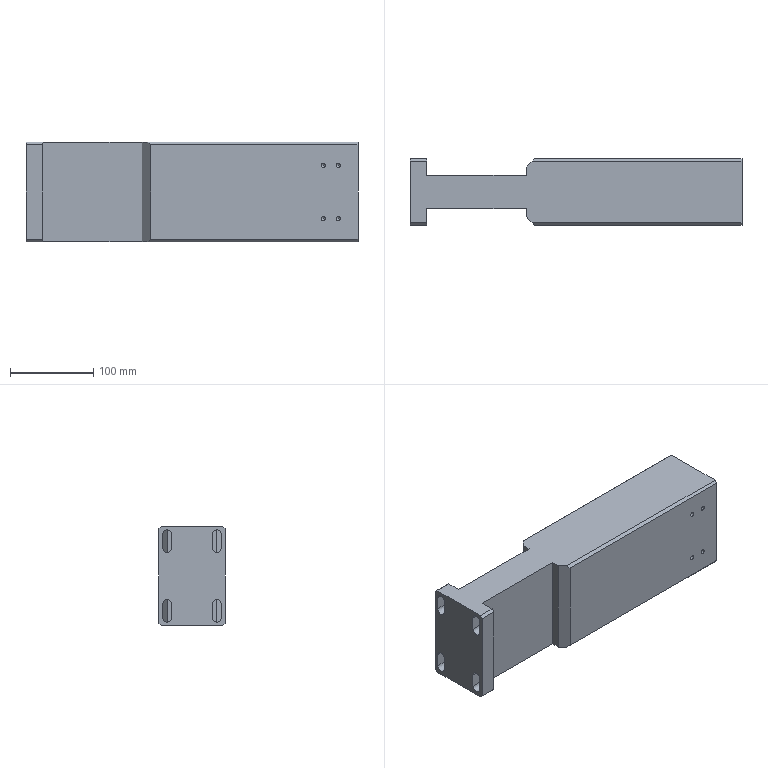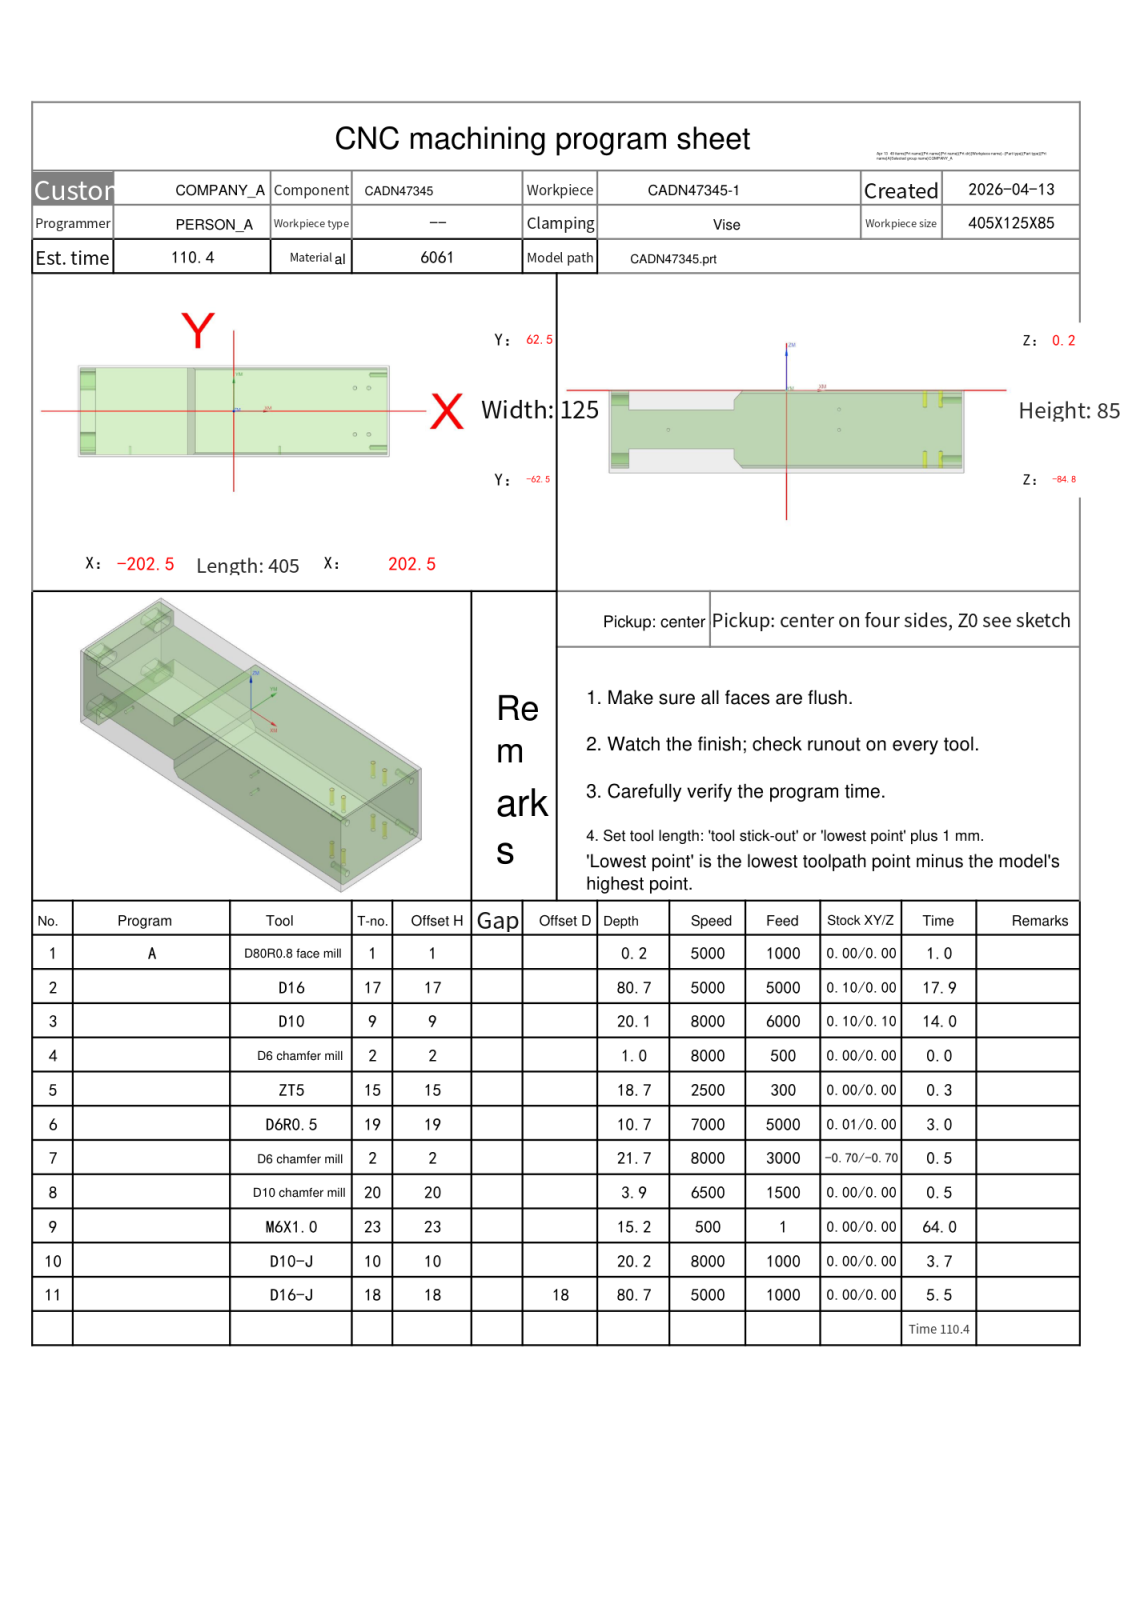NC program | NX | posted by the shop | part box 400 x 80 x 120 mm
Lines 4941 to 5986 of 5986:
N4 T02 M06
(D6 chamfer mill  D=6. R=0. H=02 ce=0.00 di=0.10)
G00 G90 G54 X158. Y32. M03 S8000
G43 H02 Z20.
M08
G98 G81 X158. Y32. Z-.8 R1. F500.
X176.
Y-32.
X158.
G80
G00 Z20.
G91 G28 Z0.0
M05
M09
G91 G28 Z0.0
M01
N5 T15 M06
(ZT5 D=5. DR_a=118 H=15)
G00 G90 G54 X158. Y32. M03 S2500
G43 H15 Z20.
M08
G98 G83 X158. Y32. Z-18.502 R1. F300. Q3.
X176.
Y-32.
X158.
G80
G00 Z20.
G91 G28 Z0.0
M05
M09
G91 G28 Z0.0
M01
N6 T19 M06
(D6R0.5  D=6. R=0.5 H=19 ce=0.01 di=0.00)
G00 G90 G54 X-52.801 Y-63.373 M03 S7000
G43 H19 Z10.788
M08
Z.415
G01 Z-.085 F5000.
Y-58.246
Y58.246
X-52.884 Y58.332 Z-.17
X-52.887 Y58.275
Y-58.275
X-52.884 Y-58.332
X-52.968 Y-58.417 Z-.255
X-52.972 Y-58.275
Y58.275
X-52.968 Y58.417
X-53.053 Y58.503 Z-.339
X-53.057 Y58.275
Y-58.275
X-53.053 Y-58.503
X-53.14 Y-58.588 Z-.424
X-53.141 Y-57.278
Y57.278
X-53.14 Y58.588
X-53.224 Y58.674 Z-.509
X-53.226 Y58.622
Y-58.622
X-53.224 Y-58.674
X-53.308 Y-58.759 Z-.594
X-53.311 Y-58.622
Y58.622
X-53.308 Y58.759
X-53.393 Y58.845 Z-.679
X-53.396 Y58.622
Y-58.622
X-53.393 Y-58.844
X-53.479 Y-58.93 Z-.764
X-53.481 Y-57.617
Y57.617
X-53.479 Y58.93
X-53.563 Y59.015 Z-.849
X-53.566 Y58.969
Y-58.969
X-53.563 Y-59.015
X-53.647 Y-59.099 Z-.933
X-53.65 Y-58.969
Y58.969
X-53.647 Y59.099
X-53.732 Y59.184 Z-1.018
X-53.735 Y58.969
Y-58.969
X-53.732 Y-59.184
X-53.819 Y-59.269 Z-1.103
X-53.82 Y-57.957
Y57.957
X-53.819 Y59.269
X-53.903 Y59.354 Z-1.188
X-53.905 Y59.316
Y-59.316
X-53.903 Y-59.354
X-53.987 Y-59.439 Z-1.273
X-53.99 Y-59.316
Y59.316
X-53.987 Y59.438
X-54.071 Y59.523 Z-1.358
X-54.075 Y59.316
Y-59.316
X-54.071 Y-59.523
X-54.158 Y-59.608 Z-1.442
X-54.16 Y-58.296
Y58.296
X-54.158 Y59.608
X-54.243 Y59.693 Z-1.527
X-54.244 Y59.663
Y-59.663
X-54.243 Y-59.693
X-54.326 Y-59.777 Z-1.612
X-54.329 Y-59.663
Y59.663
X-54.326 Y59.777
X-54.411 Y59.862 Z-1.697
X-54.414 Y59.663
Y-59.663
X-54.411 Y-59.862
X-54.497 Y-59.946 Z-1.782
X-54.499 Y-58.635
Y58.635
X-54.497 Y59.946
X-54.583 Y60.03 Z-1.867
X-54.584 Y58.72
Y-58.72
X-54.583 Y-60.03
X-54.666 Y-60.114 Z-1.952
X-54.669 Y-60.009
Y60.009
X-54.666 Y60.114
X-54.75 Y60.198 Z-2.036
X-54.754 Y60.009
Y-60.009
X-54.75 Y-60.198
X-54.836 Y-60.282 Z-2.121
X-54.838 Y-58.975
Y58.975
X-54.836 Y60.282
X-54.923 Y60.366 Z-2.206
Y59.06
Y-59.06
Y-60.366
X-55.005 Y-60.45 Z-2.291
X-55.008 Y-60.356
Y60.356
X-55.005 Y60.45
X-55.089 Y60.534 Z-2.376
X-55.093 Y60.356
Y-60.356
X-55.089 Y-60.534
X-55.175 Y-60.618 Z-2.461
X-55.178 Y-59.314
Y59.314
X-55.175 Y60.618
X-55.263 Y60.703 Z-2.546
Y59.399
Y-59.399
Y-60.703
X-55.346 Y-60.786 Z-2.63
X-55.348 Y-60.703
Y60.703
X-55.346 Y60.786
X-55.429 Y60.87 Z-2.715
X-55.432 Y60.703
Y-60.703
X-55.429 Y-60.87
X-55.514 Y-60.954 Z-2.8
X-55.517 Y-60.703
Y60.703
X-55.514 Y60.954
X-55.602 Y61.038 Z-2.885
Y59.739
Y-59.739
Y-61.038
X-55.645 Y-61.05 Z-2.927
X-55.686 Y-61.061 Z-2.97
X-55.687 Y-59.823
Y59.823
X-55.686 Y61.061
X-55.729 Y61.062 Z-3.012
X-55.771 Z-3.055
X-55.772 Y59.908
Y-59.908
X-55.771 Y-61.063
X-55.814 Z-3.097
X-55.856 Z-3.14
X-55.857 Y-59.993
Y59.993
X-55.856 Y61.063
X-55.899 Y61.064 Z-3.182
X-55.941 Z-3.224
X-55.942 Y60.
Y-60.
X-55.941 Y-61.064
X-55.984 Y-61.065 Z-3.267
X-56.026 Z-3.309
Y-60.
Y60.
Y61.065
X-56.069 Y61.066 Z-3.352
X-56.11 Z-3.394
X-56.111 Y60.
Y-60.
X-56.11 Y-61.066
X-56.154 Z-3.437
X-56.195 Y-61.067 Z-3.479
X-56.196 Y-60.
Y60.
X-56.195 Y61.067
X-56.238 Z-3.521
X-56.28 Y61.068 Z-3.564
X-56.281 Y60.
Y-60.
X-56.28 Y-61.068
X-56.323 Z-3.606
X-56.365 Y-61.069 Z-3.649
X-56.366 Y-60.
Y60.
X-56.365 Y61.069
X-56.408 Z-3.691
X-56.45 Y61.07 Z-3.734
X-56.451 Y60.
Y-60.
X-56.45 Y-61.069
X-56.493 Y-61.07 Z-3.776
X-56.534 Z-3.818
X-56.535 Y-60.
Y60.
X-56.534 Y61.07
X-56.578 Y61.071 Z-3.861
X-56.619 Z-3.903
X-56.62 Y60.
Y-60.
X-56.619 Y-61.071
X-56.663 Y-61.072 Z-3.946
X-56.704 Z-3.988
X-56.705 Y-60.
Y60.
X-56.704 Y61.072
X-56.748 Y61.073 Z-4.031
X-56.789 Z-4.073
X-56.79 Y60.
Y-60.
X-56.789 Y-61.073
X-56.832 Y-61.074 Z-4.115
X-56.874 Z-4.158
X-56.875 Y-60.
Y60.
X-56.874 Y61.074
X-56.917 Z-4.2
X-56.958 Y61.075 Z-4.243
X-56.96 Y61.05
Y-61.05
X-56.958 Y-61.075
X-57.002 Z-4.285
X-57.043 Y-61.076 Z-4.327
X-57.045 Y-61.05
Y61.05
X-57.043 Y61.076
X-57.087 Z-4.37
X-57.128 Y61.077 Z-4.412
X-57.129 Y61.05
Y-61.05
X-57.128 Y-61.077
X-57.172 Z-4.455
X-57.211 Z-4.497
X-57.212 Y-61.05
Y61.05
X-57.211 Y61.077
X-57.257 Y61.078 Z-4.54
X-57.298 Z-4.582
X-57.299 Y61.05
Y-61.05
X-57.298 Y-61.078
X-57.342 Y-61.079 Z-4.624
X-57.383 Z-4.667
X-57.384 Y-61.05
Y61.05
X-57.383 Y61.079
X-57.426 Z-4.709
X-57.467 Z-4.752
X-57.469 Y61.05
Y-61.05
X-57.467 Y-61.08
X-57.511 Z-4.794
X-57.552 Z-4.837
X-57.554 Y-61.05
Y61.05
X-57.552 Y61.08
X-57.596 Z-4.879
X-57.637 Y61.081 Z-4.921
X-57.639 Y61.05
Y-61.05
X-57.637 Y-61.081
X-57.681 Z-4.964
X-57.722 Z-5.006
X-57.723 Y-61.05
Y61.05
X-57.722 Y61.081
X-57.766 Y61.082 Z-5.049
X-57.807 Z-5.091
X-57.808 Y61.05
Y-61.05
X-57.807 Y-61.082
X-57.851 Z-5.134
X-57.892 Z-5.176
X-57.893 Y-61.05
Y61.05
X-57.892 Y61.082
X-57.936 Y61.083 Z-5.218
X-57.976 Z-5.261
X-57.978 Y61.05
Y-61.05
X-57.976 Y-61.083
X-58.02 Z-5.303
X-58.061 Y-61.084 Z-5.346
X-58.063 Y-61.05
Y61.05
X-58.061 Y61.084
X-58.105 Z-5.388
X-58.146 Z-5.431
X-58.148 Y61.05
Y-61.05
X-58.146 Y-61.084
X-58.19 Y-61.085 Z-5.473
X-58.231 Z-5.515
X-58.233 Y-61.05
Y61.05
X-58.231 Y61.085
X-58.275 Z-5.558
X-58.316 Z-5.6
X-58.317 Y61.05
Y-61.05
X-58.316 Y-61.085
X-58.36 Y-61.086 Z-5.643
X-58.4 Z-5.685
X-58.402 Y-61.05
Y61.05
X-58.401 Y61.086
X-58.445 Z-5.728
X-58.485 Z-5.77
X-58.487 Y61.05
Y-61.05
X-58.485 Y-61.086
X-58.53 Y-61.087 Z-5.812
X-58.57 Z-5.855
X-58.572 Y-61.05
Y61.05
X-58.57 Y61.087
X-58.614 Z-5.897
X-58.655 Z-5.94
X-58.657 Y61.05
Y-61.05
X-58.655 Y-61.087
X-58.699 Z-5.982
X-58.74 Z-6.025
X-58.742 Y-61.05
Y61.05
X-58.74 Y61.088
X-58.784 Z-6.067
X-58.825 Z-6.109
X-58.827 Y61.05
Y-61.05
X-58.825 Y-61.088
X-58.869 Z-6.152
X-58.91 Z-6.194
X-58.911 Y-61.05
Y61.05
X-58.91 Y61.088
X-58.954 Z-6.237
X-58.994 Z-6.279
X-58.996 Y61.05
Y-61.05
X-58.994 Y-61.088
X-59.039 Z-6.322
X-59.079 Z-6.364
X-59.081 Y-61.05
Y61.05
X-59.079 Y61.088
X-59.123 Z-6.406
X-59.164 Z-6.449
X-59.166 Y61.05
Y-61.05
X-59.164 Y-61.088
X-59.208 Z-6.491
X-59.249 Z-6.534
X-59.251 Y-61.05
Y61.05
X-59.249 Y61.088
X-59.293 Z-6.576
X-59.334 Z-6.619
X-59.336 Y61.05
Y-61.05
X-59.334 Y-61.089
X-59.378 Z-6.661
X-59.419 Z-6.703
X-59.42 Y-60.
Y61.05
X-59.419 Y61.089
X-59.463 Z-6.746
X-59.504 Z-6.788
X-59.505 Y61.05
Y-61.05
X-59.504 Y-61.089
X-59.548 Z-6.831
X-59.588 Z-6.873
X-59.59 Y-61.05
Y61.05
X-59.588 Y61.089
X-59.633 Z-6.916
X-59.673 Z-6.958
X-59.675 Y61.05
Y-61.05
X-59.673 Y-61.089
X-59.717 Z-7.
X-59.758 Z-7.043
X-59.76 Y-60.
Y61.05
X-59.758 Y61.089
X-59.802 Z-7.085
X-59.844 Z-7.128
X-59.845 Y60.
Y-60.
X-59.844 Y-61.089
X-59.887 Z-7.17
X-59.928 Z-7.212
X-59.93 Y-61.05
Y61.05
X-59.928 Y61.089
X-59.972 Z-7.255
X-60.013 Z-7.297
X-60.014 Y61.05
Y-61.05
X-60.013 Y-61.089
X-60.057 Z-7.34
X-60.097 Z-7.382
X-60.099 Y-61.05
Y61.05
X-60.097 Y61.089
X-60.142 Z-7.425
X-60.182 Z-7.467
X-60.184 Y61.05
Y-61.05
X-60.182 Y-61.089
X-60.227 Z-7.509
X-60.267 Z-7.552
X-60.269 Y-61.05
Y61.05
X-60.267 Y61.089
X-60.311 Z-7.594
X-60.352 Y61.088 Z-7.637
X-60.354 Y61.05
Y-61.05
X-60.352 Y-61.088
X-60.396 Z-7.679
X-60.437 Z-7.722
X-60.439 Y-61.05
Y61.05
X-60.437 Y61.088
X-60.481 Z-7.764
X-60.522 Z-7.806
X-60.524 Y61.05
Y-61.05
X-60.522 Y-61.088
X-60.566 Z-7.849
X-60.607 Y-61.087 Z-7.891
X-60.608 Y-61.05
Y61.05
X-60.607 Y61.088
X-60.651 Y61.087 Z-7.934
X-60.691 Z-7.976
X-60.693 Y61.05
Y-61.05
X-60.691 Y-61.087
X-60.736 Z-8.019
X-60.776 Z-8.061
X-60.778 Y-61.05
Y61.05
X-60.776 Y61.087
X-60.821 Z-8.103
X-60.861 Z-8.146
X-60.863 Y61.05
Y-61.05
X-60.861 Y-61.086
X-60.905 Z-8.188
X-60.946 Z-8.231
X-60.948 Y-61.05
Y61.05
X-60.946 Y61.086
X-60.99 Z-8.273
X-61.031 Z-8.316
X-61.033 Y61.05
Y-61.05
X-61.031 Y-61.086
X-61.075 Z-8.358
X-61.116 Z-8.4
X-61.118 Y-61.05
Y61.05
X-61.116 Y61.086
X-61.16 Z-8.443
X-61.201 Y61.085 Z-8.485
X-61.202 Y61.05
Y-61.05
X-61.201 Y-61.085
X-61.245 Z-8.528
X-61.286 Z-8.57
X-61.287 Y-61.05
Y61.05
X-61.286 Y61.085
X-61.33 Z-8.613
X-61.37 Z-8.655
X-61.372 Y61.05
Y-61.05
X-61.37 Y-61.085
X-61.415 Y-61.084 Z-8.697
X-61.455 Z-8.74
X-61.457 Y-61.05
Y61.05
X-61.455 Y61.084
X-61.499 Z-8.782
X-61.54 Z-8.825
X-61.542 Y61.05
Y-61.05
X-61.54 Y-61.084
X-61.584 Z-8.867
X-61.625 Y-61.083 Z-8.91
X-61.627 Y-61.05
Y61.05
X-61.625 Y61.083
X-61.669 Z-8.952
X-61.71 Z-8.994
X-61.712 Y61.05
Y-61.05
X-61.71 Y-61.083
X-61.754 Y-61.082 Z-9.037
X-61.795 Z-9.079
X-61.796 Y-61.05
Y61.05
X-61.795 Y61.082
X-61.839 Z-9.122
X-61.88 Y61.081 Z-9.164
X-61.881 Y61.05
Y-61.05
X-61.88 Y-61.082
X-61.924 Y-61.081 Z-9.207
X-61.965 Z-9.249
X-61.966 Y-61.05
Y61.05
X-61.965 Y61.081
X-62.008 Z-9.291
X-62.049 Y61.08 Z-9.334
X-62.051 Y61.05
Y-61.05
X-62.049 Y-61.08
X-62.093 Z-9.376
X-62.134 Z-9.419
X-62.136 Y-61.05
Y61.05
X-62.134 Y61.08
X-62.178 Y61.079 Z-9.461
X-62.219 Z-9.504
X-62.221 Y61.05
Y-61.05
X-62.219 Y-61.079
X-62.263 Z-9.546
X-62.304 Z-9.588
X-62.305 Y-61.05
Y61.05
X-62.304 Y61.079
X-62.348 Y61.078 Z-9.631
X-62.389 Z-9.673
X-62.39 Y61.05
Y-61.05
X-62.389 Y-61.078
X-62.433 Z-9.716
X-62.474 Y-61.077 Z-9.758
X-62.475 Y-61.05
Y61.05
X-62.474 Y61.078
X-62.518 Y61.077 Z-9.801
X-62.559 Z-9.843
X-62.56 Y61.05
Y-61.05
X-62.559 Y-61.077
X-62.602 Z-9.885
X-62.644 Y-61.076 Z-9.928
X-62.645 Y-61.05
Y61.05
X-62.644 Y61.076
X-62.687 Z-9.97
X-62.728 Z-10.013
X-62.73 Y61.05
Y-61.05
X-62.728 Y-61.076
X-62.772 Y-61.075 Z-10.055
X-62.813 Z-10.097
X-62.815 Y-61.05
Y61.05
X-62.813 Y61.075
X-62.857 Z-10.14
X-62.898 Z-10.182
Y-61.075
X-62.939 Y-61.074 Z-10.222
X-62.978 Z-10.262
Y61.074
X-63.019 Z-10.301
X-63.057 Z-10.341
Y-61.074
X-63.098 Y-61.073 Z-10.381
X-63.136 Z-10.421
Y61.073
X-63.177 Z-10.46
X-63.216 Z-10.5
Y-61.073
G00 Z10.788
G91 G28 Z0.0
M05
M09
G91 G28 Z0.0
M01
N7 T02 M06
(D6 chamfer mill  D=6. R=0. H=02 ce=-0.70 di=0.00)
G00 G90 G54 X175.13 Y-32.232 M03 S8000
G43 H02 Z20.
M08
Z-.8
G01 Z-1.3 F600.
X174.5 Y-32.4
G03 X176. Y-33.9 I1.5 J0.0
X177.9 Y-32. I0.0 J1.9
X176. Y-30.1 I-1.9 J0.0
X174.1 Y-32. I0.0 J-1.9
X176. Y-33.9 I1.9 J0.0
X177.5 Y-32.4 I0.0 J1.5
G01 X176.87 Y-32.232
Z-.8
G00 Z20.
X157.13
Z-.8
G01 Z-1.3
X156.5 Y-32.4
G03 X158. Y-33.9 I1.5 J0.0
X159.9 Y-32. I0.0 J1.9
X158. Y-30.1 I-1.9 J0.0
X156.1 Y-32. I0.0 J-1.9
X158. Y-33.9 I1.9 J0.0
X159.5 Y-32.4 I0.0 J1.5
G01 X158.87 Y-32.232
Z-.8
G00 Z20.
X157.13 Y31.768
Z-.8
G01 Z-1.3
X156.5 Y31.6
G03 X158. Y30.1 I1.5 J0.0
X159.9 Y32. I0.0 J1.9
X158. Y33.9 I-1.9 J0.0
X156.1 Y32. I0.0 J-1.9
X158. Y30.1 I1.9 J0.0
X159.5 Y31.6 I0.0 J1.5
G01 X158.87 Y31.768
Z-.8
G00 Z20.
X175.13
Z-.8
G01 Z-1.3
X174.5 Y31.6
G03 X176. Y30.1 I1.5 J0.0
X177.9 Y32. I0.0 J1.9
X176. Y33.9 I-1.9 J0.0
X174.1 Y32. I0.0 J-1.9
X176. Y30.1 I1.9 J0.0
X177.5 Y31.6 I0.0 J1.5
G01 X176.87 Y31.768
Z-.8
G00 Z20.
G00 G90 X-201.207 Y-57.461 M03 S8000
Z20.
Z2.935
G01 Z-1.5 F3000.
X-201.267 Y-57.289
X-201.3 Y-57.
Y57.
X-201.267 Y57.289
X-201.207 Y57.461
Z2.935
G00 Z20.
X-178.793
Z2.935
G01 Z-1.5
X-178.733 Y57.289
X-178.7 Y57.
Y0.0
Y-57.
X-178.733 Y-57.289
X-178.793 Y-57.461
Z2.935
G00 Z20.
X201.207 Y57.461
Z2.935
G01 Z-1.5
X201.267 Y57.289
X201.3 Y57.
Y-57.
X201.267 Y-57.289
X201.207 Y-57.461
Z2.935
G00 Z20.
X-63.032 Y-62.128
Z-7.184
G01 Z-21.5
G03 X-62.951 Y-61.828 I-.52 J.3
X-63.251 Y-61.308 I-.6 J0.0
G01 X-63.281 Y-61.3
X-176.719
X-176.749 Y-61.308
G03 X-177.049 Y-61.828 I.3 J-.52
X-176.968 Y-62.128 I.6 J0.0
G01 Z-.177
G00 Z20.
Y62.128
Z-.177
G01 Z-21.5
G03 X-177.049 Y61.828 I.52 J-.3
X-176.749 Y61.308 I.6 J0.0
G01 X-176.719 Y61.3
X-63.281
X-63.251 Y61.308
G03 X-62.951 Y61.828 I-.3 J.52
X-63.032 Y62.128 I-.6 J0.0
G01 Z-7.184
G00 Z20.
G91 G28 Z0.0
M05
M09
G91 G28 Z0.0
M01
N8 T20 M06
(D10 chamfer mill  D=10. R=0. H=20 ce=0.00 di=0.00)
G00 G90 G54 X-59.603 Y62.7 M03 S6500
G43 H20 Z20.
M08
Z-2.2
G01 Z-3.7 F1500.
G03 X-57.603 Y60.7 I2. J0.0
G01 X204.603
G03 X205.7 Y61.028 I0.0 J2.
G01 Z-2.2
G00 Z20.
Y-61.028
Z-2.2
G01 Z-3.7
G03 X204.603 Y-60.7 I-1.097 J-1.672
G01 X-57.603
G03 X-59.603 Y-62.7 I0.0 J-2.
G01 Z-2.2
G00 Z20.
X-174.3 Y-61.028
Z-2.2
G01 Z-3.7
G03 X-175.397 Y-60.7 I-1.097 J-1.672
G01 X-204.603
G03 X-205.7 Y-61.028 I0.0 J-2.
G01 Z-2.2
G00 Z20.
Y61.028
Z-2.2
G01 Z-3.7
G03 X-204.603 Y60.7 I1.097 J1.672
G01 X-175.397
G03 X-174.3 Y61.028 I0.0 J2.
G01 Z-2.2
G00 Z20.
G91 G28 Z0.0
M05
M09
G91 G28 Z0.0
M01
N9 T23 M06
(M6X1.0 D=5. DR_a=180 H=23)
G00 G90 G54 X158. Y32. M03 S500
G43 H23 Z20.
M08
G95
G98 G84 X158. Y32. Z-15. R1. F1. Q3.
X176.
Y-32.
X158.
G80
G94
G00 Z20.
G91 G28 Z0.0
M05
M09
G91 G28 Z0.0
M01
N10 T10 M06
(D10-J  D=10. R=0. H=10 ce=0.40 di=0.00)
G00 G90 G54 X-172.599 Y-67. M03 S8000
G43 H10 Z10.4
M08
Z-18.5
G01 Z-20. F1000.
Y-63.
G03 X-174.599 Y-65. I0.0 J-2.
G01 Y64.1
G02 X-173.699 Y65. I.9 J0.0
G01 X-170.635
G02 X-169.635 Y64. I0.0 J-1.
G01 Y-64.1
G03 X-168.735 Y-65. I.9 J0.0
G01 X-165.672
G03 X-164.672 Y-64. I0.0 J1.
G01 Y64.1
G02 X-163.772 Y65. I.9 J0.0
G01 X-160.708
G02 X-159.708 Y64. I0.0 J-1.
G01 Y-64.1
G03 X-158.808 Y-65. I.9 J0.0
G01 X-155.745
G03 X-154.745 Y-64. I0.0 J1.
G01 Y64.1
G02 X-153.845 Y65. I.9 J0.0
G01 X-150.781
G02 X-149.781 Y64. I0.0 J-1.
G01 Y-64.1
G03 X-148.881 Y-65. I.9 J0.0
G01 X-145.817
G03 X-144.817 Y-64. I0.0 J1.
G01 Y64.1
G02 X-143.917 Y65. I.9 J0.0
G01 X-140.854
G02 X-139.854 Y64. I0.0 J-1.
G01 Y-64.1
G03 X-138.954 Y-65. I.9 J0.0
G01 X-135.89
G03 X-134.89 Y-64. I0.0 J1.
G01 Y64.1
G02 X-133.99 Y65. I.9 J0.0
G01 X-130.927
G02 X-129.927 Y64. I0.0 J-1.
G01 Y-64.1
G03 X-129.027 Y-65. I.9 J0.0
G01 X-125.963
G03 X-124.963 Y-64. I0.0 J1.
G01 Y64.
G02 X-123.963 Y65. I1. J0.0
G01 X-120.9
G02 X-120. Y64.1 I0.0 J-.9
G01 Y-64.1
G03 X-119.1 Y-65. I.9 J0.0
G01 X-116.036
G03 X-115.036 Y-64. I0.0 J1.
G01 Y64.1
G02 X-114.136 Y65. I.9 J0.0
G01 X-111.072
G02 X-110.072 Y64. I0.0 J-1.
G01 Y-64.1
G03 X-109.172 Y-65. I.9 J0.0
G01 X-106.109
G03 X-105.109 Y-64. I0.0 J1.
G01 Y64.1
G02 X-104.209 Y65. I.9 J0.0
G01 X-101.145
G02 X-100.145 Y64. I0.0 J-1.
G01 Y-64.1
G03 X-99.245 Y-65. I.9 J0.0
G01 X-96.182
G03 X-95.182 Y-64. I0.0 J1.
G01 Y64.1
G02 X-94.282 Y65. I.9 J0.0
G01 X-91.218
G02 X-90.218 Y64. I0.0 J-1.
G01 Y-64.1
G03 X-89.318 Y-65. I.9 J0.0
G01 X-86.254
G03 X-85.254 Y-64. I0.0 J1.
G01 Y64.1
G02 X-84.354 Y65. I.9 J0.0
G01 X-81.291
G02 X-80.291 Y64. I0.0 J-1.
G01 Y-64.1
G03 X-79.391 Y-65. I.9 J0.0
G01 X-76.327
G03 X-75.327 Y-64. I0.0 J1.
G01 Y64.1
G02 X-74.427 Y65. I.9 J0.0
G01 X-71.364
G02 X-70.364 Y64. I0.0 J-1.
G01 Y-64.1
G03 X-69.464 Y-65. I.9 J0.0
G01 X-66.4
G03 X-65.4 Y-64. I0.0 J1.
G01 Y65.
G03 X-67.4 Y67. I-2. J0.0
G01 Z-18.5
G00 Z10.4
G00 G90 X-67.199 Y-67. M03 S8000
Z10.2
Z-9.
G01 Z-10. F1000.
G41 D10
X-66.999
G03 X-65. Y-65. I-.001 J2.
G01 Y65.
G03 X-66.999 Y67. I-2. J0.0
G01 G40 X-67.199
Z-9.
G00 X-172.801
G01 Z-10.
G41 D10
X-173.001
G03 X-175. Y65. I.001 J-2.
G01 Y-65.
G03 X-173.001 Y-67. I2. J0.0
G01 G40 X-172.801
Z-9.
G00 X-67.199
Z-19.
G01 Z-20.
G41 D10
X-66.999
G03 X-65. Y-65. I-.001 J2.
G01 Y65.
G03 X-66.999 Y67. I-2. J0.0
G01 G40 X-67.199
Z-19.
G00 X-172.801
G01 Z-20.
G41 D10
X-173.001
G03 X-175. Y65. I.001 J-2.
G01 Y-65.
G03 X-173.001 Y-67. I2. J0.0
G01 G40 X-172.801
Z-19.
G00 Z10.2
G91 G28 Z0.0
M05
M09
G91 G28 Z0.0
M01
N11 T18 M06
(D16-J  D=16. R=0. H=18 ce=0.00 di=0.00)
G00 G90 G54 X201.01 Y-69.144 M03 S5000
G43 H18 Z20.
M08
Z-15.6
G01 Z-16.1 F1000.
G41 D18
X200.998 Y-68.944
G03 X200. Y-68. I-.998 J-.056
G01 X-200.
G02 X-208. Y-60. I0.0 J8.
G01 Y60.
G02 X-200. Y68. I8. J0.0
G01 X200.
G02 X208. Y60. I0.0 J-8.
G01 Y-60.
G02 X200. Y-68. I-8. J0.0
G01 X199.5
G03 X198.5 Y-69. I0.0 J-1.
G01 G40 Y-69.2
Z-15.6
G00 Z20.
X201.01 Y-69.144
Z-31.7
G01 Z-32.2
G41 D18
X200.998 Y-68.944
G03 X200. Y-68. I-.998 J-.056
G01 X-200.
G02 X-208. Y-60. I0.0 J8.
G01 Y60.
G02 X-200. Y68. I8. J0.0
G01 X200.
G02 X208. Y60. I0.0 J-8.
G01 Y-60.
G02 X200. Y-68. I-8. J0.0
G01 X199.5
G03 X198.5 Y-69. I0.0 J-1.
G01 G40 Y-69.2
Z-31.7
G00 Z20.
X201.01 Y-69.144
Z-47.8
G01 Z-48.3
G41 D18
X200.998 Y-68.944
G03 X200. Y-68. I-.998 J-.056
G01 X-200.
G02 X-208. Y-60. I0.0 J8.
G01 Y60.
G02 X-200. Y68. I8. J0.0
G01 X200.
G02 X208. Y60. I0.0 J-8.
G01 Y-60.
G02 X200. Y-68. I-8. J0.0
G01 X199.5
G03 X198.5 Y-69. I0.0 J-1.
G01 G40 Y-69.2
Z-47.8
G00 Z20.
X201.01 Y-69.144
Z-63.9
G01 Z-64.4
G41 D18
X200.998 Y-68.944
G03 X200. Y-68. I-.998 J-.056
G01 X-200.
G02 X-208. Y-60. I0.0 J8.
G01 Y60.
G02 X-200. Y68. I8. J0.0
G01 X200.
G02 X208. Y60. I0.0 J-8.
G01 Y-60.
G02 X200. Y-68. I-8. J0.0
G01 X199.5
G03 X198.5 Y-69. I0.0 J-1.
G01 G40 Y-69.2
Z-63.9
G00 Z20.
X201.01 Y-69.144
Z-80.
G01 Z-80.5
G41 D18
X200.998 Y-68.944
G03 X200. Y-68. I-.998 J-.056
G01 X-200.
G02 X-208. Y-60. I0.0 J8.
G01 Y60.
G02 X-200. Y68. I8. J0.0
G01 X200.
G02 X208. Y60. I0.0 J-8.
G01 Y-60.
G02 X200. Y-68. I-8. J0.0
G01 X199.5
G03 X198.5 Y-69. I0.0 J-1.
G01 G40 Y-69.2
Z-80.
G00 Z20.
M05
M09
G91 G28 Z0.0
G91 G28 Y0.0
M30
%